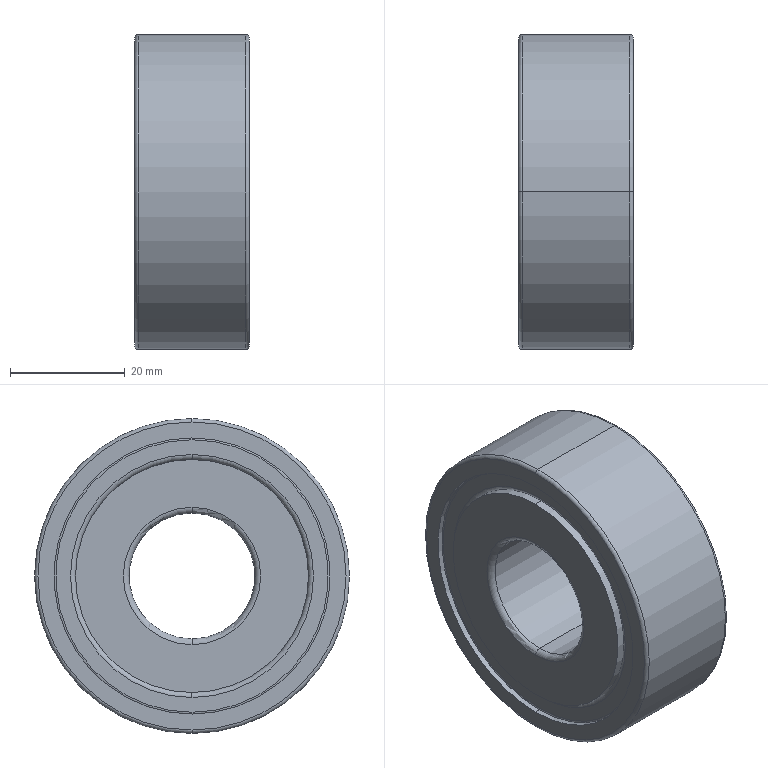Part | STEP file | Completa.sldasm-Part-108_Valor predeterminado | 1 solid | 40 faces | box 20 x 55 x 55 mm | volume 38716 mm3 | torus 16 | cylinder 16 | plane 8 | commonest cylinder face diameters 40.7 x4 48.225 x4 49.3 x4 22 x2 55 x2